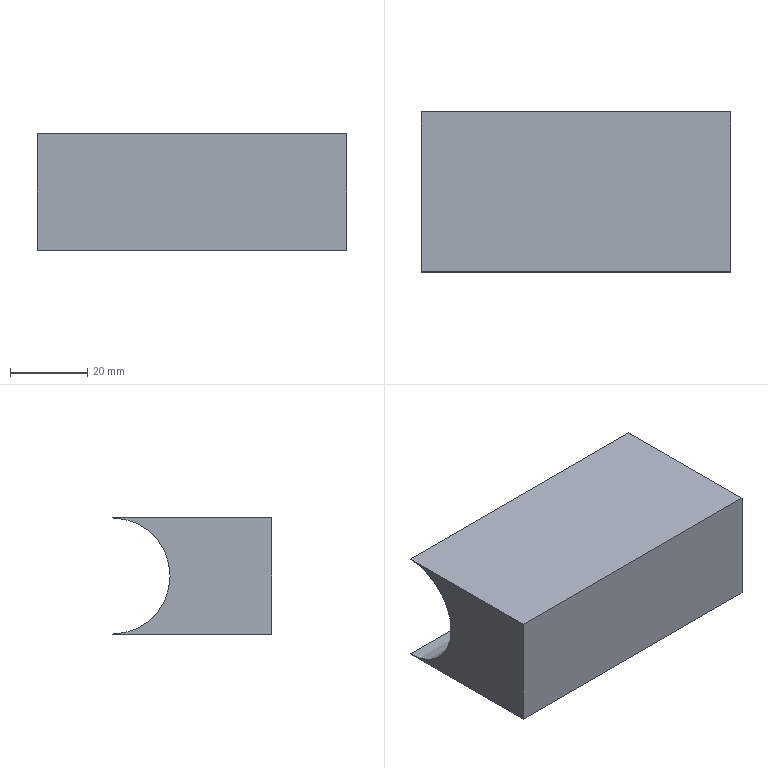Part | SolidWorks | features Extrusion 1, ICE 1 | 1 solid | 6 faces | box 80 x 41.33 x 30 mm | volume 70918 mm3 | plane 5 | cylinder 1 | commonest cylinder face diameters 30 x1
STEP:
#1=CARTESIAN_POINT('',(40.,0.,15.));
#2=VERTEX_POINT('',#1);
#3=CARTESIAN_POINT('',(40.,0.,-15.));
#4=VERTEX_POINT('',#3);
#5=CARTESIAN_POINT('',(40.,0.,-15.));
#6=DIRECTION('',(0.,0.,-1.));
#7=VECTOR('',#6,1000.);
#8=LINE('',#5,#7);
#9=EDGE_CURVE('',#2,#4,#8,.T.);
#10=ORIENTED_EDGE('',*,*,#9,.T.);
#11=CARTESIAN_POINT('',(40.,41.33,-15.));
#12=VERTEX_POINT('',#11);
#13=CARTESIAN_POINT('',(40.,10.,-15.));
#14=DIRECTION('',(0.,-1.,0.));
#15=VECTOR('',#14,1000.);
#16=LINE('',#13,#15);
#17=EDGE_CURVE('',#12,#4,#16,.T.);
#18=ORIENTED_EDGE('',*,*,#17,.F.);
#19=CARTESIAN_POINT('',(40.,41.33,15.));
#20=VERTEX_POINT('',#19);
#21=CARTESIAN_POINT('',(40.,41.33,0.));
#22=DIRECTION('',(1.,0.,0.));
#23=DIRECTION('',(0.,0.,1.));
#24=AXIS2_PLACEMENT_3D('',#21,#22,#23);
#25=CIRCLE('',#24,15.);
#26=EDGE_CURVE('',#20,#12,#25,.T.);
#27=ORIENTED_EDGE('',*,*,#26,.F.);
#28=CARTESIAN_POINT('',(40.,10.,15.));
#29=DIRECTION('',(0.,-1.,0.));
#30=VECTOR('',#29,1000.);
#31=LINE('',#28,#30);
#32=EDGE_CURVE('',#20,#2,#31,.T.);
#33=ORIENTED_EDGE('',*,*,#32,.T.);
#34=EDGE_LOOP('',(#10,#18,#27,#33));
#35=FACE_OUTER_BOUND('',#34,.T.);
#36=CARTESIAN_POINT('',(40.,10.,-15.));
#37=DIRECTION('',(-1.,0.,0.));
#38=DIRECTION('',(0.,0.,1.));
#39=AXIS2_PLACEMENT_3D('',#36,#37,#38);
#40=PLANE('',#39);
#41=ADVANCED_FACE('',(#35),#40,.F.);
#42=CARTESIAN_POINT('',(-40.,0.,-15.));
#43=VERTEX_POINT('',#42);
#44=CARTESIAN_POINT('',(-40.,0.,-15.));
#45=DIRECTION('',(-1.,0.,0.));
#46=VECTOR('',#45,1000.);
#47=LINE('',#44,#46);
#48=EDGE_CURVE('',#4,#43,#47,.T.);
#49=ORIENTED_EDGE('',*,*,#48,.T.);
#50=CARTESIAN_POINT('',(-40.,41.33,-15.));
#51=VERTEX_POINT('',#50);
#52=CARTESIAN_POINT('',(-40.,10.,-15.));
#53=DIRECTION('',(0.,-1.,0.));
#54=VECTOR('',#53,1000.);
#55=LINE('',#52,#54);
#56=EDGE_CURVE('',#51,#43,#55,.T.);
#57=ORIENTED_EDGE('',*,*,#56,.F.);
#58=CARTESIAN_POINT('',(40.,41.33,-15.));
#59=DIRECTION('',(-1.,0.,0.));
#60=VECTOR('',#59,1000.);
#61=LINE('',#58,#60);
#62=EDGE_CURVE('',#12,#51,#61,.T.);
#63=ORIENTED_EDGE('',*,*,#62,.F.);
#64=ORIENTED_EDGE('',*,*,#17,.T.);
#65=EDGE_LOOP('',(#49,#57,#63,#64));
#66=FACE_OUTER_BOUND('',#65,.T.);
#67=CARTESIAN_POINT('',(-40.,10.,-15.));
#68=DIRECTION('',(0.,0.,1.));
#69=DIRECTION('',(1.,0.,0.));
#70=AXIS2_PLACEMENT_3D('',#67,#68,#69);
#71=PLANE('',#70);
#72=ADVANCED_FACE('',(#66),#71,.F.);
#73=CARTESIAN_POINT('',(-40.,0.,15.));
#74=VERTEX_POINT('',#73);
#75=CARTESIAN_POINT('',(-40.,0.,-15.));
#76=DIRECTION('',(0.,0.,1.));
#77=VECTOR('',#76,1000.);
#78=LINE('',#75,#77);
#79=EDGE_CURVE('',#43,#74,#78,.T.);
#80=ORIENTED_EDGE('',*,*,#79,.T.);
#81=CARTESIAN_POINT('',(-40.,41.33,15.));
#82=VERTEX_POINT('',#81);
#83=CARTESIAN_POINT('',(-40.,10.,15.));
#84=DIRECTION('',(0.,-1.,0.));
#85=VECTOR('',#84,1000.);
#86=LINE('',#83,#85);
#87=EDGE_CURVE('',#82,#74,#86,.T.);
#88=ORIENTED_EDGE('',*,*,#87,.F.);
#89=CARTESIAN_POINT('',(-40.,41.33,0.));
#90=DIRECTION('',(1.,0.,0.));
#91=DIRECTION('',(0.,0.,1.));
#92=AXIS2_PLACEMENT_3D('',#89,#90,#91);
#93=CIRCLE('',#92,15.);
#94=EDGE_CURVE('',#82,#51,#93,.T.);
#95=ORIENTED_EDGE('',*,*,#94,.T.);
#96=ORIENTED_EDGE('',*,*,#56,.T.);
#97=EDGE_LOOP('',(#80,#88,#95,#96));
#98=FACE_OUTER_BOUND('',#97,.T.);
#99=CARTESIAN_POINT('',(-40.,10.,-15.));
#100=DIRECTION('',(1.,0.,0.));
#101=DIRECTION('',(0.,0.,-1.));
#102=AXIS2_PLACEMENT_3D('',#99,#100,#101);
#103=PLANE('',#102);
#104=ADVANCED_FACE('',(#98),#103,.F.);
#105=CARTESIAN_POINT('',(-40.,0.,15.));
#106=DIRECTION('',(1.,0.,0.));
#107=VECTOR('',#106,1000.);
#108=LINE('',#105,#107);
#109=EDGE_CURVE('',#74,#2,#108,.T.);
#110=ORIENTED_EDGE('',*,*,#109,.T.);
#111=ORIENTED_EDGE('',*,*,#32,.F.);
#112=CARTESIAN_POINT('',(40.,41.33,15.));
#113=DIRECTION('',(-1.,0.,0.));
#114=VECTOR('',#113,1000.);
#115=LINE('',#112,#114);
#116=EDGE_CURVE('',#20,#82,#115,.T.);
#117=ORIENTED_EDGE('',*,*,#116,.T.);
#118=ORIENTED_EDGE('',*,*,#87,.T.);
#119=EDGE_LOOP('',(#110,#111,#117,#118));
#120=FACE_OUTER_BOUND('',#119,.T.);
#121=CARTESIAN_POINT('',(-40.,10.,15.));
#122=DIRECTION('',(0.,0.,-1.));
#123=DIRECTION('',(-1.,0.,0.));
#124=AXIS2_PLACEMENT_3D('',#121,#122,#123);
#125=PLANE('',#124);
#126=ADVANCED_FACE('',(#120),#125,.F.);
#127=ORIENTED_EDGE('',*,*,#9,.F.);
#128=ORIENTED_EDGE('',*,*,#109,.F.);
#129=ORIENTED_EDGE('',*,*,#79,.F.);
#130=ORIENTED_EDGE('',*,*,#48,.F.);
#131=EDGE_LOOP('',(#127,#128,#129,#130));
#132=FACE_OUTER_BOUND('',#131,.T.);
#133=CARTESIAN_POINT('',(0.,0.,0.));
#134=DIRECTION('',(0.,1.,0.));
#135=DIRECTION('',(0.,0.,1.));
#136=AXIS2_PLACEMENT_3D('',#133,#134,#135);
#137=PLANE('',#136);
#138=ADVANCED_FACE('',(#132),#137,.F.);
#139=ORIENTED_EDGE('',*,*,#94,.F.);
#140=ORIENTED_EDGE('',*,*,#116,.F.);
#141=ORIENTED_EDGE('',*,*,#26,.T.);
#142=ORIENTED_EDGE('',*,*,#62,.T.);
#143=EDGE_LOOP('',(#139,#140,#141,#142));
#144=FACE_OUTER_BOUND('',#143,.T.);
#145=CARTESIAN_POINT('',(40.,41.33,0.));
#146=DIRECTION('',(-1.,0.,0.));
#147=DIRECTION('',(0.,0.,1.));
#148=AXIS2_PLACEMENT_3D('',#145,#146,#147);
#149=CYLINDRICAL_SURFACE('',#148,15.);
#150=ADVANCED_FACE('',(#144),#149,.F.);
#151=CLOSED_SHELL('',(#41,#72,#104,#126,#138,#150));
#152=MANIFOLD_SOLID_BREP('',#151);
#153=CARTESIAN_POINT('',(0.,0.,0.));
#154=DIRECTION('',(0.,0.,1.));
#155=DIRECTION('',(1.,0.,0.));
#156=AXIS2_PLACEMENT_3D('',#153,#154,#155);
#157=(LENGTH_UNIT()NAMED_UNIT(*)SI_UNIT(.MILLI.,.METRE.));
#158=UNCERTAINTY_MEASURE_WITH_UNIT(LENGTH_MEASURE(0.00001),#157,'','');
#159=(NAMED_UNIT(*)PLANE_ANGLE_UNIT()SI_UNIT($,.RADIAN.));
#160=(NAMED_UNIT(*)SI_UNIT($,.STERADIAN.)SOLID_ANGLE_UNIT());
#161=(GEOMETRIC_REPRESENTATION_CONTEXT(3)GLOBAL_UNCERTAINTY_ASSIGNED_CONTEXT((#158))GLOBAL_UNIT_ASSIGNED_CONTEXT((#157,#159,#160))REPRESENTATION_CONTEXT('',''));
#162=ADVANCED_BREP_SHAPE_REPRESENTATION('',(#152,#156),#161);